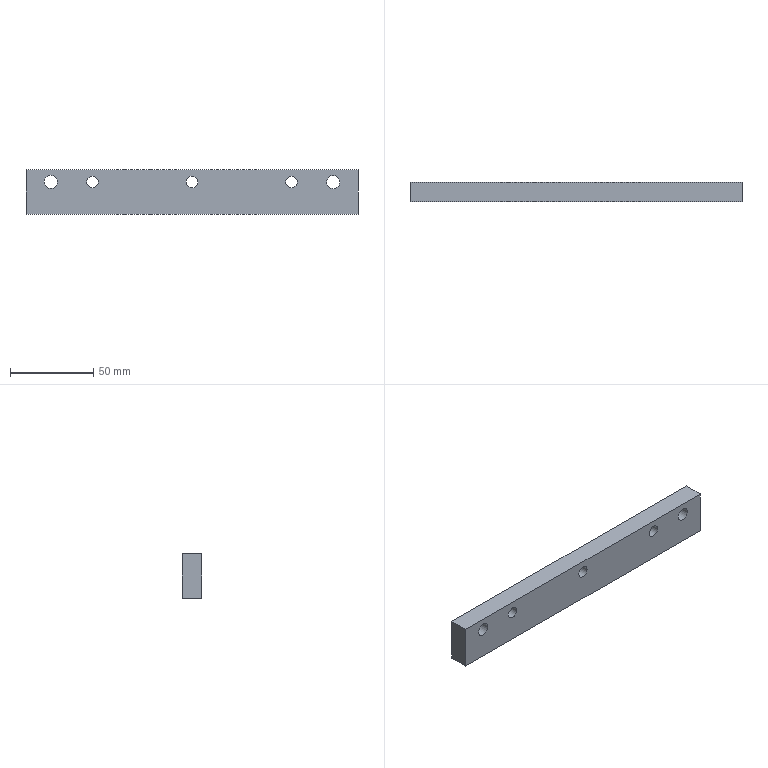Part | STEP file | SN10_001_003_GUIA | 1 solid | 17 faces | box 200 x 11.9 x 27 mm | volume 60502 mm3 | plane 9 | cylinder 8 | commonest cylinder face diameters 7 x3 11 x3 8 x2
STEP:
#1=CARTESIAN_POINT('',(0.,0.,0.));
#2=DIRECTION('',(0.,0.,1.));
#3=DIRECTION('',(1.,0.,0.));
#4=AXIS2_PLACEMENT_3D('',#1,#2,#3);
#5=CARTESIAN_POINT('',(88.51,226.9,59.418));
#6=VERTEX_POINT('',#5);
#7=CARTESIAN_POINT('',(85.,226.9,57.5));
#8=DIRECTION('',(0.,-1.,0.));
#9=DIRECTION('',(1.,0.,0.));
#10=AXIS2_PLACEMENT_3D('',#7,#8,#9);
#11=CIRCLE('',#10,4.);
#12=CARTESIAN_POINT('',(85.,226.8,57.5));
#13=DIRECTION('',(0.,-1.,0.));
#14=DIRECTION('',(0.8776,0.,0.4794));
#15=AXIS2_PLACEMENT_3D('',#12,#13,#14);
#16=CYLINDRICAL_SURFACE('',#15,4.);
#17=CARTESIAN_POINT('',(-0.5,-0.1));
#18=DIRECTION('',(1.,0.));
#19=VECTOR('',#18,1.);
#20=LINE('',#17,#19);
#21=(GEOMETRIC_REPRESENTATION_CONTEXT(2)PARAMETRIC_REPRESENTATION_CONTEXT()REPRESENTATION_CONTEXT('',''));
#22=DEFINITIONAL_REPRESENTATION('',(#20),#21);
#23=PCURVE('',#16,#22);
#24=CARTESIAN_POINT('',(0.,226.9,65.));
#25=DIRECTION('',(0.,-1.,0.));
#26=DIRECTION('',(0.,0.,-1.));
#27=AXIS2_PLACEMENT_3D('',#24,#25,#26);
#28=PLANE('',#27);
#29=CARTESIAN_POINT('',(7.5,85.));
#30=DIRECTION('',(0.,1.));
#31=AXIS2_PLACEMENT_2D('',#29,#30);
#32=CIRCLE('',#31,4.);
#33=(GEOMETRIC_REPRESENTATION_CONTEXT(2)PARAMETRIC_REPRESENTATION_CONTEXT()REPRESENTATION_CONTEXT('',''));
#34=DEFINITIONAL_REPRESENTATION('',(#32),#33);
#35=PCURVE('',#28,#34);
#36=SURFACE_CURVE('',#11,(#23,#35),.PCURVE_S1.);
#37=EDGE_CURVE('',#6,#6,#36,.T.);
#38=ORIENTED_EDGE('',*,*,#37,.T.);
#39=CARTESIAN_POINT('',(88.51,215.,59.418));
#40=VERTEX_POINT('',#39);
#41=CARTESIAN_POINT('',(88.51,226.9,59.418));
#42=CARTESIAN_POINT('',(88.51,215.,59.418));
#43=B_SPLINE_CURVE_WITH_KNOTS('',1,(#41,#42),.UNSPECIFIED.,.F.,.F.,(2,2),(-0.1,11.8),.PIECEWISE_BEZIER_KNOTS.);
#44=CARTESIAN_POINT('',(6.283,0.));
#45=DIRECTION('',(0.,1.));
#46=VECTOR('',#45,1.);
#47=LINE('',#44,#46);
#48=(GEOMETRIC_REPRESENTATION_CONTEXT(2)PARAMETRIC_REPRESENTATION_CONTEXT()REPRESENTATION_CONTEXT('',''));
#49=DEFINITIONAL_REPRESENTATION('',(#47),#48);
#50=PCURVE('',#16,#49);
#51=CARTESIAN_POINT('',(0.,0.));
#52=DIRECTION('',(0.,1.));
#53=VECTOR('',#52,1.);
#54=LINE('',#51,#53);
#55=(GEOMETRIC_REPRESENTATION_CONTEXT(2)PARAMETRIC_REPRESENTATION_CONTEXT()REPRESENTATION_CONTEXT('',''));
#56=DEFINITIONAL_REPRESENTATION('',(#54),#55);
#57=PCURVE('',#16,#56);
#58=SEAM_CURVE('',#43,(#50,#57),.PCURVE_S1.);
#59=EDGE_CURVE('',#6,#40,#58,.T.);
#60=ORIENTED_EDGE('',*,*,#59,.T.);
#61=CARTESIAN_POINT('',(85.,215.,57.5));
#62=DIRECTION('',(0.,-1.,0.));
#63=DIRECTION('',(1.,0.,0.));
#64=AXIS2_PLACEMENT_3D('',#61,#62,#63);
#65=CIRCLE('',#64,4.);
#66=CARTESIAN_POINT('',(-0.5,11.8));
#67=DIRECTION('',(1.,0.));
#68=VECTOR('',#67,1.);
#69=LINE('',#66,#68);
#70=(GEOMETRIC_REPRESENTATION_CONTEXT(2)PARAMETRIC_REPRESENTATION_CONTEXT()REPRESENTATION_CONTEXT('',''));
#71=DEFINITIONAL_REPRESENTATION('',(#69),#70);
#72=PCURVE('',#16,#71);
#73=CARTESIAN_POINT('',(0.,215.,38.));
#74=DIRECTION('',(0.,1.,0.));
#75=DIRECTION('',(0.,0.,1.));
#76=AXIS2_PLACEMENT_3D('',#73,#74,#75);
#77=PLANE('',#76);
#78=CARTESIAN_POINT('',(19.5,89.));
#79=CARTESIAN_POINT('',(26.428,89.));
#80=CARTESIAN_POINT('',(22.964,83.));
#81=CARTESIAN_POINT('',(19.5,77.));
#82=CARTESIAN_POINT('',(16.036,83.));
#83=CARTESIAN_POINT('',(12.572,89.));
#84=CARTESIAN_POINT('',(19.5,89.));
#85=(BOUNDED_CURVE()B_SPLINE_CURVE(2,(#78,#79,#80,#81,#82,#83,#84),.UNSPECIFIED.,.T.,.F.)B_SPLINE_CURVE_WITH_KNOTS((1,2,2,2,2,1),(-2.094,0.,2.094,4.189,6.283,8.378),.UNSPECIFIED.)CURVE()GEOMETRIC_REPRESENTATION_ITEM()RATIONAL_B_SPLINE_CURVE((1.,0.5,1.,0.5,1.,0.5,1.))REPRESENTATION_ITEM(''));
#86=(GEOMETRIC_REPRESENTATION_CONTEXT(2)PARAMETRIC_REPRESENTATION_CONTEXT()REPRESENTATION_CONTEXT('',''));
#87=DEFINITIONAL_REPRESENTATION('',(#85),#86);
#88=PCURVE('',#77,#87);
#89=SURFACE_CURVE('',#65,(#72,#88),.PCURVE_S1.);
#90=EDGE_CURVE('',#40,#40,#89,.T.);
#91=ORIENTED_EDGE('',*,*,#90,.F.);
#92=ORIENTED_EDGE('',*,*,#59,.F.);
#93=EDGE_LOOP('',(#38,#60,#91,#92));
#94=FACE_BOUND('',#93,.F.);
#95=ADVANCED_FACE('',(#94),#16,.F.);
#96=CARTESIAN_POINT('',(-100.,226.9,65.));
#97=VERTEX_POINT('',#96);
#98=CARTESIAN_POINT('',(100.,226.9,65.));
#99=VERTEX_POINT('',#98);
#100=CARTESIAN_POINT('',(-100.,226.9,65.));
#101=DIRECTION('',(1.,0.,0.));
#102=VECTOR('',#101,1.);
#103=LINE('',#100,#102);
#104=CARTESIAN_POINT('',(0.,215.,65.));
#105=DIRECTION('',(0.,0.,-1.));
#106=DIRECTION('',(-1.,0.,0.));
#107=AXIS2_PLACEMENT_3D('',#104,#105,#106);
#108=PLANE('',#107);
#109=CARTESIAN_POINT('',(100.,11.9));
#110=DIRECTION('',(-1.,0.));
#111=VECTOR('',#110,1.);
#112=LINE('',#109,#111);
#113=(GEOMETRIC_REPRESENTATION_CONTEXT(2)PARAMETRIC_REPRESENTATION_CONTEXT()REPRESENTATION_CONTEXT('',''));
#114=DEFINITIONAL_REPRESENTATION('',(#112),#113);
#115=PCURVE('',#108,#114);
#116=CARTESIAN_POINT('',(0.,-100.));
#117=DIRECTION('',(0.,1.));
#118=VECTOR('',#117,1.);
#119=LINE('',#116,#118);
#120=(GEOMETRIC_REPRESENTATION_CONTEXT(2)PARAMETRIC_REPRESENTATION_CONTEXT()REPRESENTATION_CONTEXT('',''));
#121=DEFINITIONAL_REPRESENTATION('',(#119),#120);
#122=PCURVE('',#28,#121);
#123=SURFACE_CURVE('',#103,(#115,#122),.PCURVE_S1.);
#124=EDGE_CURVE('',#97,#99,#123,.T.);
#125=ORIENTED_EDGE('',*,*,#124,.F.);
#126=CARTESIAN_POINT('',(-100.,215.,65.));
#127=VERTEX_POINT('',#126);
#128=CARTESIAN_POINT('',(-100.,215.,65.));
#129=DIRECTION('',(0.,1.,0.));
#130=VECTOR('',#129,1.);
#131=LINE('',#128,#130);
#132=CARTESIAN_POINT('',(100.,0.));
#133=DIRECTION('',(0.,1.));
#134=VECTOR('',#133,1.);
#135=LINE('',#132,#134);
#136=(GEOMETRIC_REPRESENTATION_CONTEXT(2)PARAMETRIC_REPRESENTATION_CONTEXT()REPRESENTATION_CONTEXT('',''));
#137=DEFINITIONAL_REPRESENTATION('',(#135),#136);
#138=PCURVE('',#108,#137);
#139=CARTESIAN_POINT('',(-100.,0.,0.));
#140=DIRECTION('',(1.,0.,0.));
#141=DIRECTION('',(0.,0.,-1.));
#142=AXIS2_PLACEMENT_3D('',#139,#140,#141);
#143=PLANE('',#142);
#144=CARTESIAN_POINT('',(-65.,215.));
#145=DIRECTION('',(0.,1.));
#146=VECTOR('',#145,1.);
#147=LINE('',#144,#146);
#148=(GEOMETRIC_REPRESENTATION_CONTEXT(2)PARAMETRIC_REPRESENTATION_CONTEXT()REPRESENTATION_CONTEXT('',''));
#149=DEFINITIONAL_REPRESENTATION('',(#147),#148);
#150=PCURVE('',#143,#149);
#151=SURFACE_CURVE('',#131,(#138,#150),.PCURVE_S1.);
#152=EDGE_CURVE('',#127,#97,#151,.T.);
#153=ORIENTED_EDGE('',*,*,#152,.F.);
#154=CARTESIAN_POINT('',(100.,215.,65.));
#155=VERTEX_POINT('',#154);
#156=CARTESIAN_POINT('',(-100.,215.,65.));
#157=DIRECTION('',(1.,0.,0.));
#158=VECTOR('',#157,1.);
#159=LINE('',#156,#158);
#160=CARTESIAN_POINT('',(100.,0.));
#161=DIRECTION('',(-1.,0.));
#162=VECTOR('',#161,1.);
#163=LINE('',#160,#162);
#164=(GEOMETRIC_REPRESENTATION_CONTEXT(2)PARAMETRIC_REPRESENTATION_CONTEXT()REPRESENTATION_CONTEXT('',''));
#165=DEFINITIONAL_REPRESENTATION('',(#163),#164);
#166=PCURVE('',#108,#165);
#167=CARTESIAN_POINT('',(27.,-100.));
#168=DIRECTION('',(0.,1.));
#169=VECTOR('',#168,1.);
#170=LINE('',#167,#169);
#171=(GEOMETRIC_REPRESENTATION_CONTEXT(2)PARAMETRIC_REPRESENTATION_CONTEXT()REPRESENTATION_CONTEXT('',''));
#172=DEFINITIONAL_REPRESENTATION('',(#170),#171);
#173=PCURVE('',#77,#172);
#174=SURFACE_CURVE('',#159,(#166,#173),.PCURVE_S1.);
#175=EDGE_CURVE('',#127,#155,#174,.T.);
#176=ORIENTED_EDGE('',*,*,#175,.T.);
#177=CARTESIAN_POINT('',(100.,215.,65.));
#178=DIRECTION('',(0.,1.,0.));
#179=VECTOR('',#178,1.);
#180=LINE('',#177,#179);
#181=CARTESIAN_POINT('',(-100.,0.));
#182=DIRECTION('',(0.,1.));
#183=VECTOR('',#182,1.);
#184=LINE('',#181,#183);
#185=(GEOMETRIC_REPRESENTATION_CONTEXT(2)PARAMETRIC_REPRESENTATION_CONTEXT()REPRESENTATION_CONTEXT('',''));
#186=DEFINITIONAL_REPRESENTATION('',(#184),#185);
#187=PCURVE('',#108,#186);
#188=CARTESIAN_POINT('',(100.,0.,0.));
#189=DIRECTION('',(1.,0.,0.));
#190=DIRECTION('',(0.,0.,-1.));
#191=AXIS2_PLACEMENT_3D('',#188,#189,#190);
#192=PLANE('',#191);
#193=CARTESIAN_POINT('',(-65.,215.));
#194=DIRECTION('',(0.,1.));
#195=VECTOR('',#194,1.);
#196=LINE('',#193,#195);
#197=(GEOMETRIC_REPRESENTATION_CONTEXT(2)PARAMETRIC_REPRESENTATION_CONTEXT()REPRESENTATION_CONTEXT('',''));
#198=DEFINITIONAL_REPRESENTATION('',(#196),#197);
#199=PCURVE('',#192,#198);
#200=SURFACE_CURVE('',#180,(#187,#199),.PCURVE_S1.);
#201=EDGE_CURVE('',#155,#99,#200,.T.);
#202=ORIENTED_EDGE('',*,*,#201,.T.);
#203=EDGE_LOOP('',(#125,#153,#176,#202));
#204=FACE_BOUND('',#203,.T.);
#205=ADVANCED_FACE('',(#204),#108,.F.);
#206=CARTESIAN_POINT('',(-100.,226.9,38.));
#207=VERTEX_POINT('',#206);
#208=CARTESIAN_POINT('',(-100.,226.9,65.));
#209=DIRECTION('',(0.,0.,-1.));
#210=VECTOR('',#209,1.);
#211=LINE('',#208,#210);
#212=CARTESIAN_POINT('',(-65.,226.9));
#213=DIRECTION('',(1.,0.));
#214=VECTOR('',#213,1.);
#215=LINE('',#212,#214);
#216=(GEOMETRIC_REPRESENTATION_CONTEXT(2)PARAMETRIC_REPRESENTATION_CONTEXT()REPRESENTATION_CONTEXT('',''));
#217=DEFINITIONAL_REPRESENTATION('',(#215),#216);
#218=PCURVE('',#143,#217);
#219=CARTESIAN_POINT('',(0.,-100.));
#220=DIRECTION('',(1.,0.));
#221=VECTOR('',#220,1.);
#222=LINE('',#219,#221);
#223=(GEOMETRIC_REPRESENTATION_CONTEXT(2)PARAMETRIC_REPRESENTATION_CONTEXT()REPRESENTATION_CONTEXT('',''));
#224=DEFINITIONAL_REPRESENTATION('',(#222),#223);
#225=PCURVE('',#28,#224);
#226=SURFACE_CURVE('',#211,(#218,#225),.PCURVE_S1.);
#227=EDGE_CURVE('',#97,#207,#226,.T.);
#228=ORIENTED_EDGE('',*,*,#227,.T.);
#229=CARTESIAN_POINT('',(-100.,215.,38.));
#230=VERTEX_POINT('',#229);
#231=CARTESIAN_POINT('',(-100.,226.9,38.));
#232=DIRECTION('',(0.,-1.,0.));
#233=VECTOR('',#232,1.);
#234=LINE('',#231,#233);
#235=CARTESIAN_POINT('',(-38.,226.9));
#236=DIRECTION('',(0.,-1.));
#237=VECTOR('',#236,1.);
#238=LINE('',#235,#237);
#239=(GEOMETRIC_REPRESENTATION_CONTEXT(2)PARAMETRIC_REPRESENTATION_CONTEXT()REPRESENTATION_CONTEXT('',''));
#240=DEFINITIONAL_REPRESENTATION('',(#238),#239);
#241=PCURVE('',#143,#240);
#242=CARTESIAN_POINT('',(0.,226.9,38.));
#243=DIRECTION('',(0.,0.,1.));
#244=DIRECTION('',(1.,0.,0.));
#245=AXIS2_PLACEMENT_3D('',#242,#243,#244);
#246=PLANE('',#245);
#247=CARTESIAN_POINT('',(-100.,0.));
#248=DIRECTION('',(0.,-1.));
#249=VECTOR('',#248,1.);
#250=LINE('',#247,#249);
#251=(GEOMETRIC_REPRESENTATION_CONTEXT(2)PARAMETRIC_REPRESENTATION_CONTEXT()REPRESENTATION_CONTEXT('',''));
#252=DEFINITIONAL_REPRESENTATION('',(#250),#251);
#253=PCURVE('',#246,#252);
#254=SURFACE_CURVE('',#234,(#241,#253),.PCURVE_S1.);
#255=EDGE_CURVE('',#207,#230,#254,.T.);
#256=ORIENTED_EDGE('',*,*,#255,.T.);
#257=CARTESIAN_POINT('',(-100.,215.,38.));
#258=DIRECTION('',(0.,0.,1.));
#259=VECTOR('',#258,1.);
#260=LINE('',#257,#259);
#261=CARTESIAN_POINT('',(-38.,215.));
#262=DIRECTION('',(-1.,0.));
#263=VECTOR('',#262,1.);
#264=LINE('',#261,#263);
#265=(GEOMETRIC_REPRESENTATION_CONTEXT(2)PARAMETRIC_REPRESENTATION_CONTEXT()REPRESENTATION_CONTEXT('',''));
#266=DEFINITIONAL_REPRESENTATION('',(#264),#265);
#267=PCURVE('',#143,#266);
#268=CARTESIAN_POINT('',(0.,-100.));
#269=DIRECTION('',(1.,0.));
#270=VECTOR('',#269,1.);
#271=LINE('',#268,#270);
#272=(GEOMETRIC_REPRESENTATION_CONTEXT(2)PARAMETRIC_REPRESENTATION_CONTEXT()REPRESENTATION_CONTEXT('',''));
#273=DEFINITIONAL_REPRESENTATION('',(#271),#272);
#274=PCURVE('',#77,#273);
#275=SURFACE_CURVE('',#260,(#267,#274),.PCURVE_S1.);
#276=EDGE_CURVE('',#230,#127,#275,.T.);
#277=ORIENTED_EDGE('',*,*,#276,.T.);
#278=ORIENTED_EDGE('',*,*,#152,.T.);
#279=EDGE_LOOP('',(#228,#256,#277,#278));
#280=FACE_BOUND('',#279,.T.);
#281=ADVANCED_FACE('',(#280),#143,.F.);
#282=CARTESIAN_POINT('',(55.173,226.9,54.863));
#283=VERTEX_POINT('',#282);
#284=CARTESIAN_POINT('',(60.,226.9,57.5));
#285=DIRECTION('',(0.,-1.,0.));
#286=DIRECTION('',(1.,0.,0.));
#287=AXIS2_PLACEMENT_3D('',#284,#285,#286);
#288=CIRCLE('',#287,5.5);
#289=CARTESIAN_POINT('',(60.,226.8,57.5));
#290=DIRECTION('',(0.,-1.,0.));
#291=DIRECTION('',(0.8776,0.,0.4794));
#292=AXIS2_PLACEMENT_3D('',#289,#290,#291);
#293=CYLINDRICAL_SURFACE('',#292,5.5);
#294=CARTESIAN_POINT('',(-0.5,-0.1));
#295=DIRECTION('',(1.,0.));
#296=VECTOR('',#295,1.);
#297=LINE('',#294,#296);
#298=(GEOMETRIC_REPRESENTATION_CONTEXT(2)PARAMETRIC_REPRESENTATION_CONTEXT()REPRESENTATION_CONTEXT('',''));
#299=DEFINITIONAL_REPRESENTATION('',(#297),#298);
#300=PCURVE('',#293,#299);
#301=CARTESIAN_POINT('',(7.5,60.));
#302=DIRECTION('',(0.,1.));
#303=AXIS2_PLACEMENT_2D('',#301,#302);
#304=CIRCLE('',#303,5.5);
#305=(GEOMETRIC_REPRESENTATION_CONTEXT(2)PARAMETRIC_REPRESENTATION_CONTEXT()REPRESENTATION_CONTEXT('',''));
#306=DEFINITIONAL_REPRESENTATION('',(#304),#305);
#307=PCURVE('',#28,#306);
#308=SURFACE_CURVE('',#288,(#300,#307),.PCURVE_S1.);
#309=EDGE_CURVE('',#283,#283,#308,.T.);
#310=ORIENTED_EDGE('',*,*,#309,.T.);
#311=CARTESIAN_POINT('',(55.173,219.9,54.863));
#312=VERTEX_POINT('',#311);
#313=CARTESIAN_POINT('',(55.173,226.9,54.863));
#314=CARTESIAN_POINT('',(55.173,219.9,54.863));
#315=B_SPLINE_CURVE_WITH_KNOTS('',1,(#313,#314),.UNSPECIFIED.,.F.,.F.,(2,2),(-0.1,6.9),.PIECEWISE_BEZIER_KNOTS.);
#316=CARTESIAN_POINT('',(9.425,0.));
#317=DIRECTION('',(0.,1.));
#318=VECTOR('',#317,1.);
#319=LINE('',#316,#318);
#320=(GEOMETRIC_REPRESENTATION_CONTEXT(2)PARAMETRIC_REPRESENTATION_CONTEXT()REPRESENTATION_CONTEXT('',''));
#321=DEFINITIONAL_REPRESENTATION('',(#319),#320);
#322=PCURVE('',#293,#321);
#323=CARTESIAN_POINT('',(3.142,0.));
#324=DIRECTION('',(0.,1.));
#325=VECTOR('',#324,1.);
#326=LINE('',#323,#325);
#327=(GEOMETRIC_REPRESENTATION_CONTEXT(2)PARAMETRIC_REPRESENTATION_CONTEXT()REPRESENTATION_CONTEXT('',''));
#328=DEFINITIONAL_REPRESENTATION('',(#326),#327);
#329=PCURVE('',#293,#328);
#330=SEAM_CURVE('',#315,(#322,#329),.PCURVE_S1.);
#331=EDGE_CURVE('',#283,#312,#330,.T.);
#332=ORIENTED_EDGE('',*,*,#331,.T.);
#333=CARTESIAN_POINT('',(60.,219.9,57.5));
#334=DIRECTION('',(0.,-1.,0.));
#335=DIRECTION('',(1.,0.,0.));
#336=AXIS2_PLACEMENT_3D('',#333,#334,#335);
#337=CIRCLE('',#336,5.5);
#338=CARTESIAN_POINT('',(-0.5,6.9));
#339=DIRECTION('',(1.,0.));
#340=VECTOR('',#339,1.);
#341=LINE('',#338,#340);
#342=(GEOMETRIC_REPRESENTATION_CONTEXT(2)PARAMETRIC_REPRESENTATION_CONTEXT()REPRESENTATION_CONTEXT('',''));
#343=DEFINITIONAL_REPRESENTATION('',(#341),#342);
#344=PCURVE('',#293,#343);
#345=CARTESIAN_POINT('',(63.5,219.9,57.5));
#346=DIRECTION('',(0.,-1.,0.));
#347=DIRECTION('',(0.,0.,-1.));
#348=AXIS2_PLACEMENT_3D('',#345,#346,#347);
#349=PLANE('',#348);
#350=CARTESIAN_POINT('',(0.,-3.5));
#351=DIRECTION('',(0.,1.));
#352=AXIS2_PLACEMENT_2D('',#350,#351);
#353=CIRCLE('',#352,5.5);
#354=(GEOMETRIC_REPRESENTATION_CONTEXT(2)PARAMETRIC_REPRESENTATION_CONTEXT()REPRESENTATION_CONTEXT('',''));
#355=DEFINITIONAL_REPRESENTATION('',(#353),#354);
#356=PCURVE('',#349,#355);
#357=SURFACE_CURVE('',#337,(#344,#356),.PCURVE_S1.);
#358=EDGE_CURVE('',#312,#312,#357,.T.);
#359=ORIENTED_EDGE('',*,*,#358,.F.);
#360=ORIENTED_EDGE('',*,*,#331,.F.);
#361=EDGE_LOOP('',(#310,#332,#359,#360));
#362=FACE_BOUND('',#361,.F.);
#363=ADVANCED_FACE('',(#362),#293,.F.);
#364=CARTESIAN_POINT('',(-4.827,226.9,54.863));
#365=VERTEX_POINT('',#364);
#366=CARTESIAN_POINT('',(0.,226.9,57.5));
#367=DIRECTION('',(0.,-1.,0.));
#368=DIRECTION('',(1.,0.,0.));
#369=AXIS2_PLACEMENT_3D('',#366,#367,#368);
#370=CIRCLE('',#369,5.5);
#371=CARTESIAN_POINT('',(0.,226.8,57.5));
#372=DIRECTION('',(0.,-1.,0.));
#373=DIRECTION('',(0.8776,0.,0.4794));
#374=AXIS2_PLACEMENT_3D('',#371,#372,#373);
#375=CYLINDRICAL_SURFACE('',#374,5.5);
#376=CARTESIAN_POINT('',(-0.5,-0.1));
#377=DIRECTION('',(1.,0.));
#378=VECTOR('',#377,1.);
#379=LINE('',#376,#378);
#380=(GEOMETRIC_REPRESENTATION_CONTEXT(2)PARAMETRIC_REPRESENTATION_CONTEXT()REPRESENTATION_CONTEXT('',''));
#381=DEFINITIONAL_REPRESENTATION('',(#379),#380);
#382=PCURVE('',#375,#381);
#383=CARTESIAN_POINT('',(7.5,0.));
#384=DIRECTION('',(0.,1.));
#385=AXIS2_PLACEMENT_2D('',#383,#384);
#386=CIRCLE('',#385,5.5);
#387=(GEOMETRIC_REPRESENTATION_CONTEXT(2)PARAMETRIC_REPRESENTATION_CONTEXT()REPRESENTATION_CONTEXT('',''));
#388=DEFINITIONAL_REPRESENTATION('',(#386),#387);
#389=PCURVE('',#28,#388);
#390=SURFACE_CURVE('',#370,(#382,#389),.PCURVE_S1.);
#391=EDGE_CURVE('',#365,#365,#390,.T.);
#392=ORIENTED_EDGE('',*,*,#391,.T.);
#393=CARTESIAN_POINT('',(-4.827,219.9,54.863));
#394=VERTEX_POINT('',#393);
#395=CARTESIAN_POINT('',(-4.827,226.9,54.863));
#396=CARTESIAN_POINT('',(-4.827,219.9,54.863));
#397=B_SPLINE_CURVE_WITH_KNOTS('',1,(#395,#396),.UNSPECIFIED.,.F.,.F.,(2,2),(-0.1,6.9),.PIECEWISE_BEZIER_KNOTS.);
#398=CARTESIAN_POINT('',(9.425,0.));
#399=DIRECTION('',(0.,1.));
#400=VECTOR('',#399,1.);
#401=LINE('',#398,#400);
#402=(GEOMETRIC_REPRESENTATION_CONTEXT(2)PARAMETRIC_REPRESENTATION_CONTEXT()REPRESENTATION_CONTEXT('',''));
#403=DEFINITIONAL_REPRESENTATION('',(#401),#402);
#404=PCURVE('',#375,#403);
#405=CARTESIAN_POINT('',(3.142,0.));
#406=DIRECTION('',(0.,1.));
#407=VECTOR('',#406,1.);
#408=LINE('',#405,#407);
#409=(GEOMETRIC_REPRESENTATION_CONTEXT(2)PARAMETRIC_REPRESENTATION_CONTEXT()REPRESENTATION_CONTEXT('',''));
#410=DEFINITIONAL_REPRESENTATION('',(#408),#409);
#411=PCURVE('',#375,#410);
#412=SEAM_CURVE('',#397,(#404,#411),.PCURVE_S1.);
#413=EDGE_CURVE('',#365,#394,#412,.T.);
#414=ORIENTED_EDGE('',*,*,#413,.T.);
#415=CARTESIAN_POINT('',(0.,219.9,57.5));
#416=DIRECTION('',(0.,-1.,0.));
#417=DIRECTION('',(1.,0.,0.));
#418=AXIS2_PLACEMENT_3D('',#415,#416,#417);
#419=CIRCLE('',#418,5.5);
#420=CARTESIAN_POINT('',(-0.5,6.9));
#421=DIRECTION('',(1.,0.));
#422=VECTOR('',#421,1.);
#423=LINE('',#420,#422);
#424=(GEOMETRIC_REPRESENTATION_CONTEXT(2)PARAMETRIC_REPRESENTATION_CONTEXT()REPRESENTATION_CONTEXT('',''));
#425=DEFINITIONAL_REPRESENTATION('',(#423),#424);
#426=PCURVE('',#375,#425);
#427=CARTESIAN_POINT('',(63.5,219.9,57.5));
#428=DIRECTION('',(0.,-1.,0.));
#429=DIRECTION('',(0.,0.,-1.));
#430=AXIS2_PLACEMENT_3D('',#427,#428,#429);
#431=PLANE('',#430);
#432=CARTESIAN_POINT('',(0.,-63.5));
#433=DIRECTION('',(0.,1.));
#434=AXIS2_PLACEMENT_2D('',#432,#433);
#435=CIRCLE('',#434,5.5);
#436=(GEOMETRIC_REPRESENTATION_CONTEXT(2)PARAMETRIC_REPRESENTATION_CONTEXT()REPRESENTATION_CONTEXT('',''));
#437=DEFINITIONAL_REPRESENTATION('',(#435),#436);
#438=PCURVE('',#431,#437);
#439=SURFACE_CURVE('',#419,(#426,#438),.PCURVE_S1.);
#440=EDGE_CURVE('',#394,#394,#439,.T.);
#441=ORIENTED_EDGE('',*,*,#440,.F.);
#442=ORIENTED_EDGE('',*,*,#413,.F.);
#443=EDGE_LOOP('',(#392,#414,#441,#442));
#444=FACE_BOUND('',#443,.F.);
#445=ADVANCED_FACE('',(#444),#375,.F.);
#446=CARTESIAN_POINT('',(-64.827,226.9,54.863));
#447=VERTEX_POINT('',#446);
#448=CARTESIAN_POINT('',(-60.,226.9,57.5));
#449=DIRECTION('',(0.,-1.,0.));
#450=DIRECTION('',(1.,0.,0.));
#451=AXIS2_PLACEMENT_3D('',#448,#449,#450);
#452=CIRCLE('',#451,5.5);
#453=CARTESIAN_POINT('',(-60.,226.8,57.5));
#454=DIRECTION('',(0.,-1.,0.));
#455=DIRECTION('',(0.8776,0.,0.4794));
#456=AXIS2_PLACEMENT_3D('',#453,#454,#455);
#457=CYLINDRICAL_SURFACE('',#456,5.5);
#458=CARTESIAN_POINT('',(-0.5,-0.1));
#459=DIRECTION('',(1.,0.));
#460=VECTOR('',#459,1.);
#461=LINE('',#458,#460);
#462=(GEOMETRIC_REPRESENTATION_CONTEXT(2)PARAMETRIC_REPRESENTATION_CONTEXT()REPRESENTATION_CONTEXT('',''));
#463=DEFINITIONAL_REPRESENTATION('',(#461),#462);
#464=PCURVE('',#457,#463);
#465=CARTESIAN_POINT('',(7.5,-60.));
#466=DIRECTION('',(0.,1.));
#467=AXIS2_PLACEMENT_2D('',#465,#466);
#468=CIRCLE('',#467,5.5);
#469=(GEOMETRIC_REPRESENTATION_CONTEXT(2)PARAMETRIC_REPRESENTATION_CONTEXT()REPRESENTATION_CONTEXT('',''));
#470=DEFINITIONAL_REPRESENTATION('',(#468),#469);
#471=PCURVE('',#28,#470);
#472=SURFACE_CURVE('',#452,(#464,#471),.PCURVE_S1.);
#473=EDGE_CURVE('',#447,#447,#472,.T.);
#474=ORIENTED_EDGE('',*,*,#473,.T.);
#475=CARTESIAN_POINT('',(-64.827,219.9,54.863));
#476=VERTEX_POINT('',#475);
#477=CARTESIAN_POINT('',(-64.827,226.9,54.863));
#478=CARTESIAN_POINT('',(-64.827,219.9,54.863));
#479=B_SPLINE_CURVE_WITH_KNOTS('',1,(#477,#478),.UNSPECIFIED.,.F.,.F.,(2,2),(-0.1,6.9),.PIECEWISE_BEZIER_KNOTS.);
#480=CARTESIAN_POINT('',(9.425,0.));
#481=DIRECTION('',(0.,1.));
#482=VECTOR('',#481,1.);
#483=LINE('',#480,#482);
#484=(GEOMETRIC_REPRESENTATION_CONTEXT(2)PARAMETRIC_REPRESENTATION_CONTEXT()REPRESENTATION_CONTEXT('',''));
#485=DEFINITIONAL_REPRESENTATION('',(#483),#484);
#486=PCURVE('',#457,#485);
#487=CARTESIAN_POINT('',(3.142,0.));
#488=DIRECTION('',(0.,1.));
#489=VECTOR('',#488,1.);
#490=LINE('',#487,#489);
#491=(GEOMETRIC_REPRESENTATION_CONTEXT(2)PARAMETRIC_REPRESENTATION_CONTEXT()REPRESENTATION_CONTEXT('',''));
#492=DEFINITIONAL_REPRESENTATION('',(#490),#491);
#493=PCURVE('',#457,#492);
#494=SEAM_CURVE('',#479,(#486,#493),.PCURVE_S1.);
#495=EDGE_CURVE('',#447,#476,#494,.T.);
#496=ORIENTED_EDGE('',*,*,#495,.T.);
#497=CARTESIAN_POINT('',(-60.,219.9,57.5));
#498=DIRECTION('',(0.,-1.,0.));
#499=DIRECTION('',(1.,0.,0.));
#500=AXIS2_PLACEMENT_3D('',#497,#498,#499);
#501=CIRCLE('',#500,5.5);
#502=CARTESIAN_POINT('',(-0.5,6.9));
#503=DIRECTION('',(1.,0.));
#504=VECTOR('',#503,1.);
#505=LINE('',#502,#504);
#506=(GEOMETRIC_REPRESENTATION_CONTEXT(2)PARAMETRIC_REPRESENTATION_CONTEXT()REPRESENTATION_CONTEXT('',''));
#507=DEFINITIONAL_REPRESENTATION('',(#505),#506);
#508=PCURVE('',#457,#507);
#509=CARTESIAN_POINT('',(63.5,219.9,57.5));
#510=DIRECTION('',(0.,-1.,0.));
#511=DIRECTION('',(0.,0.,-1.));
#512=AXIS2_PLACEMENT_3D('',#509,#510,#511);
#513=PLANE('',#512);
#514=CARTESIAN_POINT('',(0.,-123.5));
#515=DIRECTION('',(0.,1.));
#516=AXIS2_PLACEMENT_2D('',#514,#515);
#517=CIRCLE('',#516,5.5);
#518=(GEOMETRIC_REPRESENTATION_CONTEXT(2)PARAMETRIC_REPRESENTATION_CONTEXT()REPRESENTATION_CONTEXT('',''));
#519=DEFINITIONAL_REPRESENTATION('',(#517),#518);
#520=PCURVE('',#513,#519);
#521=SURFACE_CURVE('',#501,(#508,#520),.PCURVE_S1.);
#522=EDGE_CURVE('',#476,#476,#521,.T.);
#523=ORIENTED_EDGE('',*,*,#522,.F.);
#524=ORIENTED_EDGE('',*,*,#495,.F.);
#525=EDGE_LOOP('',(#474,#496,#523,#524));
#526=FACE_BOUND('',#525,.F.);
#527=ADVANCED_FACE('',(#526),#457,.F.);
#528=ORIENTED_EDGE('',*,*,#358,.F.);
#529=EDGE_LOOP('',(#528));
#530=FACE_BOUND('',#529,.T.);
#531=CARTESIAN_POINT('',(63.072,219.9,59.178));
#532=VERTEX_POINT('',#531);
#533=CARTESIAN_POINT('',(60.,219.9,57.5));
#534=DIRECTION('',(0.,-1.,0.));
#535=DIRECTION('',(1.,0.,0.));
#536=AXIS2_PLACEMENT_3D('',#533,#534,#535);
#537=CIRCLE('',#536,3.5);
#538=CARTESIAN_POINT('',(0.,-3.5));
#539=DIRECTION('',(0.,1.));
#540=AXIS2_PLACEMENT_2D('',#538,#539);
#541=CIRCLE('',#540,3.5);
#542=(GEOMETRIC_REPRESENTATION_CONTEXT(2)PARAMETRIC_REPRESENTATION_CONTEXT()REPRESENTATION_CONTEXT('',''));
#543=DEFINITIONAL_REPRESENTATION('',(#541),#542);
#544=PCURVE('',#349,#543);
#545=CARTESIAN_POINT('',(60.,226.8,57.5));
#546=DIRECTION('',(0.,-1.,0.));
#547=DIRECTION('',(0.8776,0.,0.4794));
#548=AXIS2_PLACEMENT_3D('',#545,#546,#547);
#549=CYLINDRICAL_SURFACE('',#548,3.5);
#550=CARTESIAN_POINT('',(-0.5,6.9));
#551=DIRECTION('',(1.,0.));
#552=VECTOR('',#551,1.);
#553=LINE('',#550,#552);
#554=(GEOMETRIC_REPRESENTATION_CONTEXT(2)PARAMETRIC_REPRESENTATION_CONTEXT()REPRESENTATION_CONTEXT('',''));
#555=DEFINITIONAL_REPRESENTATION('',(#553),#554);
#556=PCURVE('',#549,#555);
#557=SURFACE_CURVE('',#537,(#544,#556),.PCURVE_S1.);
#558=EDGE_CURVE('',#532,#532,#557,.T.);
#559=ORIENTED_EDGE('',*,*,#558,.T.);
#560=EDGE_LOOP('',(#559));
#561=FACE_BOUND('',#560,.T.);
#562=ADVANCED_FACE('',(#530,#561),#349,.F.);
#563=ORIENTED_EDGE('',*,*,#440,.F.);
#564=EDGE_LOOP('',(#563));
#565=FACE_BOUND('',#564,.T.);
#566=CARTESIAN_POINT('',(3.072,219.9,59.178));
#567=VERTEX_POINT('',#566);
#568=CARTESIAN_POINT('',(0.,219.9,57.5));
#569=DIRECTION('',(0.,-1.,0.));
#570=DIRECTION('',(1.,0.,0.));
#571=AXIS2_PLACEMENT_3D('',#568,#569,#570);
#572=CIRCLE('',#571,3.5);
#573=CARTESIAN_POINT('',(0.,-63.5));
#574=DIRECTION('',(0.,1.));
#575=AXIS2_PLACEMENT_2D('',#573,#574);
#576=CIRCLE('',#575,3.5);
#577=(GEOMETRIC_REPRESENTATION_CONTEXT(2)PARAMETRIC_REPRESENTATION_CONTEXT()REPRESENTATION_CONTEXT('',''));
#578=DEFINITIONAL_REPRESENTATION('',(#576),#577);
#579=PCURVE('',#431,#578);
#580=CARTESIAN_POINT('',(0.,226.8,57.5));
#581=DIRECTION('',(0.,-1.,0.));
#582=DIRECTION('',(0.8776,0.,0.4794));
#583=AXIS2_PLACEMENT_3D('',#580,#581,#582);
#584=CYLINDRICAL_SURFACE('',#583,3.5);
#585=CARTESIAN_POINT('',(-0.5,6.9));
#586=DIRECTION('',(1.,0.));
#587=VECTOR('',#586,1.);
#588=LINE('',#585,#587);
#589=(GEOMETRIC_REPRESENTATION_CONTEXT(2)PARAMETRIC_REPRESENTATION_CONTEXT()REPRESENTATION_CONTEXT('',''));
#590=DEFINITIONAL_REPRESENTATION('',(#588),#589);
#591=PCURVE('',#584,#590);
#592=SURFACE_CURVE('',#572,(#579,#591),.PCURVE_S1.);
#593=EDGE_CURVE('',#567,#567,#592,.T.);
#594=ORIENTED_EDGE('',*,*,#593,.T.);
#595=EDGE_LOOP('',(#594));
#596=FACE_BOUND('',#595,.T.);
#597=ADVANCED_FACE('',(#565,#596),#431,.F.);
#598=ORIENTED_EDGE('',*,*,#522,.F.);
#599=EDGE_LOOP('',(#598));
#600=FACE_BOUND('',#599,.T.);
#601=CARTESIAN_POINT('',(-56.928,219.9,59.178));
#602=VERTEX_POINT('',#601);
#603=CARTESIAN_POINT('',(-60.,219.9,57.5));
#604=DIRECTION('',(0.,-1.,0.));
#605=DIRECTION('',(1.,0.,0.));
#606=AXIS2_PLACEMENT_3D('',#603,#604,#605);
#607=CIRCLE('',#606,3.5);
#608=CARTESIAN_POINT('',(0.,-123.5));
#609=DIRECTION('',(0.,1.));
#610=AXIS2_PLACEMENT_2D('',#608,#609);
#611=CIRCLE('',#610,3.5);
#612=(GEOMETRIC_REPRESENTATION_CONTEXT(2)PARAMETRIC_REPRESENTATION_CONTEXT()REPRESENTATION_CONTEXT('',''));
#613=DEFINITIONAL_REPRESENTATION('',(#611),#612);
#614=PCURVE('',#513,#613);
#615=CARTESIAN_POINT('',(-60.,226.8,57.5));
#616=DIRECTION('',(0.,-1.,0.));
#617=DIRECTION('',(0.8776,0.,0.4794));
#618=AXIS2_PLACEMENT_3D('',#615,#616,#617);
#619=CYLINDRICAL_SURFACE('',#618,3.5);
#620=CARTESIAN_POINT('',(-0.5,6.9));
#621=DIRECTION('',(1.,0.));
#622=VECTOR('',#621,1.);
#623=LINE('',#620,#622);
#624=(GEOMETRIC_REPRESENTATION_CONTEXT(2)PARAMETRIC_REPRESENTATION_CONTEXT()REPRESENTATION_CONTEXT('',''));
#625=DEFINITIONAL_REPRESENTATION('',(#623),#624);
#626=PCURVE('',#619,#625);
#627=SURFACE_CURVE('',#607,(#614,#626),.PCURVE_S1.);
#628=EDGE_CURVE('',#602,#602,#627,.T.);
#629=ORIENTED_EDGE('',*,*,#628,.T.);
#630=EDGE_LOOP('',(#629));
#631=FACE_BOUND('',#630,.T.);
#632=ADVANCED_FACE('',(#600,#631),#513,.F.);
#633=CARTESIAN_POINT('',(63.072,215.,59.178));
#634=VERTEX_POINT('',#633);
#635=CARTESIAN_POINT('',(60.,215.,57.5));
#636=DIRECTION('',(0.,-1.,0.));
#637=DIRECTION('',(1.,0.,0.));
#638=AXIS2_PLACEMENT_3D('',#635,#636,#637);
#639=CIRCLE('',#638,3.5);
#640=CARTESIAN_POINT('',(-0.5,11.8));
#641=DIRECTION('',(1.,0.));
#642=VECTOR('',#641,1.);
#643=LINE('',#640,#642);
#644=(GEOMETRIC_REPRESENTATION_CONTEXT(2)PARAMETRIC_REPRESENTATION_CONTEXT()REPRESENTATION_CONTEXT('',''));
#645=DEFINITIONAL_REPRESENTATION('',(#643),#644);
#646=PCURVE('',#549,#645);
#647=CARTESIAN_POINT('',(19.5,63.5));
#648=CARTESIAN_POINT('',(25.562,63.5));
#649=CARTESIAN_POINT('',(22.531,58.25));
#650=CARTESIAN_POINT('',(19.5,53.));
#651=CARTESIAN_POINT('',(16.469,58.25));
#652=CARTESIAN_POINT('',(13.438,63.5));
#653=CARTESIAN_POINT('',(19.5,63.5));
#654=(BOUNDED_CURVE()B_SPLINE_CURVE(2,(#647,#648,#649,#650,#651,#652,#653),.UNSPECIFIED.,.T.,.F.)B_SPLINE_CURVE_WITH_KNOTS((1,2,2,2,2,1),(-2.094,0.,2.094,4.189,6.283,8.378),.UNSPECIFIED.)CURVE()GEOMETRIC_REPRESENTATION_ITEM()RATIONAL_B_SPLINE_CURVE((1.,0.5,1.,0.5,1.,0.5,1.))REPRESENTATION_ITEM(''));
#655=(GEOMETRIC_REPRESENTATION_CONTEXT(2)PARAMETRIC_REPRESENTATION_CONTEXT()REPRESENTATION_CONTEXT('',''));
#656=DEFINITIONAL_REPRESENTATION('',(#654),#655);
#657=PCURVE('',#77,#656);
#658=SURFACE_CURVE('',#639,(#646,#657),.PCURVE_S1.);
#659=EDGE_CURVE('',#634,#634,#658,.T.);
#660=ORIENTED_EDGE('',*,*,#659,.F.);
#661=CARTESIAN_POINT('',(63.072,219.9,59.178));
#662=CARTESIAN_POINT('',(63.072,215.,59.178));
#663=B_SPLINE_CURVE_WITH_KNOTS('',1,(#661,#662),.UNSPECIFIED.,.F.,.F.,(2,2),(6.9,11.8),.PIECEWISE_BEZIER_KNOTS.);
#664=CARTESIAN_POINT('',(0.,0.));
#665=DIRECTION('',(0.,1.));
#666=VECTOR('',#665,1.);
#667=LINE('',#664,#666);
#668=(GEOMETRIC_REPRESENTATION_CONTEXT(2)PARAMETRIC_REPRESENTATION_CONTEXT()REPRESENTATION_CONTEXT('',''));
#669=DEFINITIONAL_REPRESENTATION('',(#667),#668);
#670=PCURVE('',#549,#669);
#671=CARTESIAN_POINT('',(6.283,0.));
#672=DIRECTION('',(0.,1.));
#673=VECTOR('',#672,1.);
#674=LINE('',#671,#673);
#675=(GEOMETRIC_REPRESENTATION_CONTEXT(2)PARAMETRIC_REPRESENTATION_CONTEXT()REPRESENTATION_CONTEXT('',''));
#676=DEFINITIONAL_REPRESENTATION('',(#674),#675);
#677=PCURVE('',#549,#676);
#678=SEAM_CURVE('',#663,(#670,#677),.PCURVE_S1.);
#679=EDGE_CURVE('',#532,#634,#678,.T.);
#680=ORIENTED_EDGE('',*,*,#679,.F.);
#681=ORIENTED_EDGE('',*,*,#558,.T.);
#682=ORIENTED_EDGE('',*,*,#679,.T.);
#683=EDGE_LOOP('',(#660,#680,#681,#682));
#684=FACE_BOUND('',#683,.F.);
#685=ADVANCED_FACE('',(#684),#549,.F.);
#686=CARTESIAN_POINT('',(3.072,215.,59.178));
#687=VERTEX_POINT('',#686);
#688=CARTESIAN_POINT('',(0.,215.,57.5));
#689=DIRECTION('',(0.,-1.,0.));
#690=DIRECTION('',(1.,0.,0.));
#691=AXIS2_PLACEMENT_3D('',#688,#689,#690);
#692=CIRCLE('',#691,3.5);
#693=CARTESIAN_POINT('',(-0.5,11.8));
#694=DIRECTION('',(1.,0.));
#695=VECTOR('',#694,1.);
#696=LINE('',#693,#695);
#697=(GEOMETRIC_REPRESENTATION_CONTEXT(2)PARAMETRIC_REPRESENTATION_CONTEXT()REPRESENTATION_CONTEXT('',''));
#698=DEFINITIONAL_REPRESENTATION('',(#696),#697);
#699=PCURVE('',#584,#698);
#700=CARTESIAN_POINT('',(19.5,3.5));
#701=CARTESIAN_POINT('',(25.562,3.5));
#702=CARTESIAN_POINT('',(22.531,-1.75));
#703=CARTESIAN_POINT('',(19.5,-7.));
#704=CARTESIAN_POINT('',(16.469,-1.75));
#705=CARTESIAN_POINT('',(13.438,3.5));
#706=CARTESIAN_POINT('',(19.5,3.5));
#707=(BOUNDED_CURVE()B_SPLINE_CURVE(2,(#700,#701,#702,#703,#704,#705,#706),.UNSPECIFIED.,.T.,.F.)B_SPLINE_CURVE_WITH_KNOTS((1,2,2,2,2,1),(-2.094,0.,2.094,4.189,6.283,8.378),.UNSPECIFIED.)CURVE()GEOMETRIC_REPRESENTATION_ITEM()RATIONAL_B_SPLINE_CURVE((1.,0.5,1.,0.5,1.,0.5,1.))REPRESENTATION_ITEM(''));
#708=(GEOMETRIC_REPRESENTATION_CONTEXT(2)PARAMETRIC_REPRESENTATION_CONTEXT()REPRESENTATION_CONTEXT('',''));
#709=DEFINITIONAL_REPRESENTATION('',(#707),#708);
#710=PCURVE('',#77,#709);
#711=SURFACE_CURVE('',#692,(#699,#710),.PCURVE_S1.);
#712=EDGE_CURVE('',#687,#687,#711,.T.);
#713=ORIENTED_EDGE('',*,*,#712,.F.);
#714=CARTESIAN_POINT('',(3.072,219.9,59.178));
#715=CARTESIAN_POINT('',(3.072,215.,59.178));
#716=B_SPLINE_CURVE_WITH_KNOTS('',1,(#714,#715),.UNSPECIFIED.,.F.,.F.,(2,2),(6.9,11.8),.PIECEWISE_BEZIER_KNOTS.);
#717=CARTESIAN_POINT('',(0.,0.));
#718=DIRECTION('',(0.,1.));
#719=VECTOR('',#718,1.);
#720=LINE('',#717,#719);
#721=(GEOMETRIC_REPRESENTATION_CONTEXT(2)PARAMETRIC_REPRESENTATION_CONTEXT()REPRESENTATION_CONTEXT('',''));
#722=DEFINITIONAL_REPRESENTATION('',(#720),#721);
#723=PCURVE('',#584,#722);
#724=CARTESIAN_POINT('',(6.283,0.));
#725=DIRECTION('',(0.,1.));
#726=VECTOR('',#725,1.);
#727=LINE('',#724,#726);
#728=(GEOMETRIC_REPRESENTATION_CONTEXT(2)PARAMETRIC_REPRESENTATION_CONTEXT()REPRESENTATION_CONTEXT('',''));
#729=DEFINITIONAL_REPRESENTATION('',(#727),#728);
#730=PCURVE('',#584,#729);
#731=SEAM_CURVE('',#716,(#723,#730),.PCURVE_S1.);
#732=EDGE_CURVE('',#567,#687,#731,.T.);
#733=ORIENTED_EDGE('',*,*,#732,.F.);
#734=ORIENTED_EDGE('',*,*,#593,.T.);
#735=ORIENTED_EDGE('',*,*,#732,.T.);
#736=EDGE_LOOP('',(#713,#733,#734,#735));
#737=FACE_BOUND('',#736,.F.);
#738=ADVANCED_FACE('',(#737),#584,.F.);
#739=CARTESIAN_POINT('',(-56.928,215.,59.178));
#740=VERTEX_POINT('',#739);
#741=CARTESIAN_POINT('',(-60.,215.,57.5));
#742=DIRECTION('',(0.,-1.,0.));
#743=DIRECTION('',(1.,0.,0.));
#744=AXIS2_PLACEMENT_3D('',#741,#742,#743);
#745=CIRCLE('',#744,3.5);
#746=CARTESIAN_POINT('',(-0.5,11.8));
#747=DIRECTION('',(1.,0.));
#748=VECTOR('',#747,1.);
#749=LINE('',#746,#748);
#750=(GEOMETRIC_REPRESENTATION_CONTEXT(2)PARAMETRIC_REPRESENTATION_CONTEXT()REPRESENTATION_CONTEXT('',''));
#751=DEFINITIONAL_REPRESENTATION('',(#749),#750);
#752=PCURVE('',#619,#751);
#753=CARTESIAN_POINT('',(19.5,-56.5));
#754=CARTESIAN_POINT('',(25.562,-56.5));
#755=CARTESIAN_POINT('',(22.531,-61.75));
#756=CARTESIAN_POINT('',(19.5,-67.));
#757=CARTESIAN_POINT('',(16.469,-61.75));
#758=CARTESIAN_POINT('',(13.438,-56.5));
#759=CARTESIAN_POINT('',(19.5,-56.5));
#760=(BOUNDED_CURVE()B_SPLINE_CURVE(2,(#753,#754,#755,#756,#757,#758,#759),.UNSPECIFIED.,.T.,.F.)B_SPLINE_CURVE_WITH_KNOTS((1,2,2,2,2,1),(-2.094,0.,2.094,4.189,6.283,8.378),.UNSPECIFIED.)CURVE()GEOMETRIC_REPRESENTATION_ITEM()RATIONAL_B_SPLINE_CURVE((1.,0.5,1.,0.5,1.,0.5,1.))REPRESENTATION_ITEM(''));
#761=(GEOMETRIC_REPRESENTATION_CONTEXT(2)PARAMETRIC_REPRESENTATION_CONTEXT()REPRESENTATION_CONTEXT('',''));
#762=DEFINITIONAL_REPRESENTATION('',(#760),#761);
#763=PCURVE('',#77,#762);
#764=SURFACE_CURVE('',#745,(#752,#763),.PCURVE_S1.);
#765=EDGE_CURVE('',#740,#740,#764,.T.);
#766=ORIENTED_EDGE('',*,*,#765,.F.);
#767=CARTESIAN_POINT('',(-56.928,219.9,59.178));
#768=CARTESIAN_POINT('',(-56.928,215.,59.178));
#769=B_SPLINE_CURVE_WITH_KNOTS('',1,(#767,#768),.UNSPECIFIED.,.F.,.F.,(2,2),(6.9,11.8),.PIECEWISE_BEZIER_KNOTS.);
#770=CARTESIAN_POINT('',(0.,0.));
#771=DIRECTION('',(0.,1.));
#772=VECTOR('',#771,1.);
#773=LINE('',#770,#772);
#774=(GEOMETRIC_REPRESENTATION_CONTEXT(2)PARAMETRIC_REPRESENTATION_CONTEXT()REPRESENTATION_CONTEXT('',''));
#775=DEFINITIONAL_REPRESENTATION('',(#773),#774);
#776=PCURVE('',#619,#775);
#777=CARTESIAN_POINT('',(6.283,0.));
#778=DIRECTION('',(0.,1.));
#779=VECTOR('',#778,1.);
#780=LINE('',#777,#779);
#781=(GEOMETRIC_REPRESENTATION_CONTEXT(2)PARAMETRIC_REPRESENTATION_CONTEXT()REPRESENTATION_CONTEXT('',''));
#782=DEFINITIONAL_REPRESENTATION('',(#780),#781);
#783=PCURVE('',#619,#782);
#784=SEAM_CURVE('',#769,(#776,#783),.PCURVE_S1.);
#785=EDGE_CURVE('',#602,#740,#784,.T.);
#786=ORIENTED_EDGE('',*,*,#785,.F.);
#787=ORIENTED_EDGE('',*,*,#628,.T.);
#788=ORIENTED_EDGE('',*,*,#785,.T.);
#789=EDGE_LOOP('',(#766,#786,#787,#788));
#790=FACE_BOUND('',#789,.F.);
#791=ADVANCED_FACE('',(#790),#619,.F.);
#792=CARTESIAN_POINT('',(100.,215.,38.));
#793=VERTEX_POINT('',#792);
#794=CARTESIAN_POINT('',(-100.,215.,38.));
#795=DIRECTION('',(1.,0.,0.));
#796=VECTOR('',#795,1.);
#797=LINE('',#794,#796);
#798=CARTESIAN_POINT('',(-100.,-11.9));
#799=DIRECTION('',(1.,0.));
#800=VECTOR('',#799,1.);
#801=LINE('',#798,#800);
#802=(GEOMETRIC_REPRESENTATION_CONTEXT(2)PARAMETRIC_REPRESENTATION_CONTEXT()REPRESENTATION_CONTEXT('',''));
#803=DEFINITIONAL_REPRESENTATION('',(#801),#802);
#804=PCURVE('',#246,#803);
#805=CARTESIAN_POINT('',(0.,-100.));
#806=DIRECTION('',(0.,1.));
#807=VECTOR('',#806,1.);
#808=LINE('',#805,#807);
#809=(GEOMETRIC_REPRESENTATION_CONTEXT(2)PARAMETRIC_REPRESENTATION_CONTEXT()REPRESENTATION_CONTEXT('',''));
#810=DEFINITIONAL_REPRESENTATION('',(#808),#809);
#811=PCURVE('',#77,#810);
#812=SURFACE_CURVE('',#797,(#804,#811),.PCURVE_S1.);
#813=EDGE_CURVE('',#230,#793,#812,.T.);
#814=ORIENTED_EDGE('',*,*,#813,.F.);
#815=ORIENTED_EDGE('',*,*,#255,.F.);
#816=CARTESIAN_POINT('',(100.,226.9,38.));
#817=VERTEX_POINT('',#816);
#818=CARTESIAN_POINT('',(-100.,226.9,38.));
#819=DIRECTION('',(1.,0.,0.));
#820=VECTOR('',#819,1.);
#821=LINE('',#818,#820);
#822=CARTESIAN_POINT('',(-100.,0.));
#823=DIRECTION('',(1.,0.));
#824=VECTOR('',#823,1.);
#825=LINE('',#822,#824);
#826=(GEOMETRIC_REPRESENTATION_CONTEXT(2)PARAMETRIC_REPRESENTATION_CONTEXT()REPRESENTATION_CONTEXT('',''));
#827=DEFINITIONAL_REPRESENTATION('',(#825),#826);
#828=PCURVE('',#246,#827);
#829=CARTESIAN_POINT('',(27.,-100.));
#830=DIRECTION('',(0.,1.));
#831=VECTOR('',#830,1.);
#832=LINE('',#829,#831);
#833=(GEOMETRIC_REPRESENTATION_CONTEXT(2)PARAMETRIC_REPRESENTATION_CONTEXT()REPRESENTATION_CONTEXT('',''));
#834=DEFINITIONAL_REPRESENTATION('',(#832),#833);
#835=PCURVE('',#28,#834);
#836=SURFACE_CURVE('',#821,(#828,#835),.PCURVE_S1.);
#837=EDGE_CURVE('',#207,#817,#836,.T.);
#838=ORIENTED_EDGE('',*,*,#837,.T.);
#839=CARTESIAN_POINT('',(100.,226.9,38.));
#840=DIRECTION('',(0.,-1.,0.));
#841=VECTOR('',#840,1.);
#842=LINE('',#839,#841);
#843=CARTESIAN_POINT('',(100.,0.));
#844=DIRECTION('',(0.,-1.));
#845=VECTOR('',#844,1.);
#846=LINE('',#843,#845);
#847=(GEOMETRIC_REPRESENTATION_CONTEXT(2)PARAMETRIC_REPRESENTATION_CONTEXT()REPRESENTATION_CONTEXT('',''));
#848=DEFINITIONAL_REPRESENTATION('',(#846),#847);
#849=PCURVE('',#246,#848);
#850=CARTESIAN_POINT('',(-38.,226.9));
#851=DIRECTION('',(0.,-1.));
#852=VECTOR('',#851,1.);
#853=LINE('',#850,#852);
#854=(GEOMETRIC_REPRESENTATION_CONTEXT(2)PARAMETRIC_REPRESENTATION_CONTEXT()REPRESENTATION_CONTEXT('',''));
#855=DEFINITIONAL_REPRESENTATION('',(#853),#854);
#856=PCURVE('',#192,#855);
#857=SURFACE_CURVE('',#842,(#849,#856),.PCURVE_S1.);
#858=EDGE_CURVE('',#817,#793,#857,.T.);
#859=ORIENTED_EDGE('',*,*,#858,.T.);
#860=EDGE_LOOP('',(#814,#815,#838,#859));
#861=FACE_BOUND('',#860,.T.);
#862=ADVANCED_FACE('',(#861),#246,.F.);
#863=ORIENTED_EDGE('',*,*,#201,.F.);
#864=CARTESIAN_POINT('',(100.,215.,38.));
#865=DIRECTION('',(0.,0.,1.));
#866=VECTOR('',#865,1.);
#867=LINE('',#864,#866);
#868=CARTESIAN_POINT('',(-38.,215.));
#869=DIRECTION('',(-1.,0.));
#870=VECTOR('',#869,1.);
#871=LINE('',#868,#870);
#872=(GEOMETRIC_REPRESENTATION_CONTEXT(2)PARAMETRIC_REPRESENTATION_CONTEXT()REPRESENTATION_CONTEXT('',''));
#873=DEFINITIONAL_REPRESENTATION('',(#871),#872);
#874=PCURVE('',#192,#873);
#875=CARTESIAN_POINT('',(0.,100.));
#876=DIRECTION('',(1.,0.));
#877=VECTOR('',#876,1.);
#878=LINE('',#875,#877);
#879=(GEOMETRIC_REPRESENTATION_CONTEXT(2)PARAMETRIC_REPRESENTATION_CONTEXT()REPRESENTATION_CONTEXT('',''));
#880=DEFINITIONAL_REPRESENTATION('',(#878),#879);
#881=PCURVE('',#77,#880);
#882=SURFACE_CURVE('',#867,(#874,#881),.PCURVE_S1.);
#883=EDGE_CURVE('',#793,#155,#882,.T.);
#884=ORIENTED_EDGE('',*,*,#883,.F.);
#885=ORIENTED_EDGE('',*,*,#858,.F.);
#886=CARTESIAN_POINT('',(100.,226.9,65.));
#887=DIRECTION('',(0.,0.,-1.));
#888=VECTOR('',#887,1.);
#889=LINE('',#886,#888);
#890=CARTESIAN_POINT('',(-65.,226.9));
#891=DIRECTION('',(1.,0.));
#892=VECTOR('',#891,1.);
#893=LINE('',#890,#892);
#894=(GEOMETRIC_REPRESENTATION_CONTEXT(2)PARAMETRIC_REPRESENTATION_CONTEXT()REPRESENTATION_CONTEXT('',''));
#895=DEFINITIONAL_REPRESENTATION('',(#893),#894);
#896=PCURVE('',#192,#895);
#897=CARTESIAN_POINT('',(0.,100.));
#898=DIRECTION('',(1.,0.));
#899=VECTOR('',#898,1.);
#900=LINE('',#897,#899);
#901=(GEOMETRIC_REPRESENTATION_CONTEXT(2)PARAMETRIC_REPRESENTATION_CONTEXT()REPRESENTATION_CONTEXT('',''));
#902=DEFINITIONAL_REPRESENTATION('',(#900),#901);
#903=PCURVE('',#28,#902);
#904=SURFACE_CURVE('',#889,(#896,#903),.PCURVE_S1.);
#905=EDGE_CURVE('',#99,#817,#904,.T.);
#906=ORIENTED_EDGE('',*,*,#905,.F.);
#907=EDGE_LOOP('',(#863,#884,#885,#906));
#908=FACE_BOUND('',#907,.T.);
#909=ADVANCED_FACE('',(#908),#192,.T.);
#910=ORIENTED_EDGE('',*,*,#837,.F.);
#911=ORIENTED_EDGE('',*,*,#227,.F.);
#912=ORIENTED_EDGE('',*,*,#124,.T.);
#913=ORIENTED_EDGE('',*,*,#905,.T.);
#914=EDGE_LOOP('',(#910,#911,#912,#913));
#915=FACE_BOUND('',#914,.T.);
#916=CARTESIAN_POINT('',(-81.49,226.9,59.418));
#917=VERTEX_POINT('',#916);
#918=CARTESIAN_POINT('',(-85.,226.9,57.5));
#919=DIRECTION('',(0.,-1.,0.));
#920=DIRECTION('',(1.,0.,0.));
#921=AXIS2_PLACEMENT_3D('',#918,#919,#920);
#922=CIRCLE('',#921,4.);
#923=CARTESIAN_POINT('',(7.5,-85.));
#924=DIRECTION('',(0.,1.));
#925=AXIS2_PLACEMENT_2D('',#923,#924);
#926=CIRCLE('',#925,4.);
#927=(GEOMETRIC_REPRESENTATION_CONTEXT(2)PARAMETRIC_REPRESENTATION_CONTEXT()REPRESENTATION_CONTEXT('',''));
#928=DEFINITIONAL_REPRESENTATION('',(#926),#927);
#929=PCURVE('',#28,#928);
#930=CARTESIAN_POINT('',(-85.,226.8,57.5));
#931=DIRECTION('',(0.,-1.,0.));
#932=DIRECTION('',(0.8776,0.,0.4794));
#933=AXIS2_PLACEMENT_3D('',#930,#931,#932);
#934=CYLINDRICAL_SURFACE('',#933,4.);
#935=CARTESIAN_POINT('',(-0.5,-0.1));
#936=DIRECTION('',(1.,0.));
#937=VECTOR('',#936,1.);
#938=LINE('',#935,#937);
#939=(GEOMETRIC_REPRESENTATION_CONTEXT(2)PARAMETRIC_REPRESENTATION_CONTEXT()REPRESENTATION_CONTEXT('',''));
#940=DEFINITIONAL_REPRESENTATION('',(#938),#939);
#941=PCURVE('',#934,#940);
#942=SURFACE_CURVE('',#922,(#929,#941),.PCURVE_S1.);
#943=EDGE_CURVE('',#917,#917,#942,.T.);
#944=ORIENTED_EDGE('',*,*,#943,.T.);
#945=EDGE_LOOP('',(#944));
#946=FACE_BOUND('',#945,.T.);
#947=ORIENTED_EDGE('',*,*,#37,.T.);
#948=EDGE_LOOP('',(#947));
#949=FACE_BOUND('',#948,.T.);
#950=ORIENTED_EDGE('',*,*,#309,.T.);
#951=EDGE_LOOP('',(#950));
#952=FACE_BOUND('',#951,.T.);
#953=ORIENTED_EDGE('',*,*,#391,.T.);
#954=EDGE_LOOP('',(#953));
#955=FACE_BOUND('',#954,.T.);
#956=ORIENTED_EDGE('',*,*,#473,.T.);
#957=EDGE_LOOP('',(#956));
#958=FACE_BOUND('',#957,.T.);
#959=ADVANCED_FACE('',(#915,#946,#949,#952,#955,#958),#28,.F.);
#960=ORIENTED_EDGE('',*,*,#175,.F.);
#961=ORIENTED_EDGE('',*,*,#276,.F.);
#962=ORIENTED_EDGE('',*,*,#813,.T.);
#963=ORIENTED_EDGE('',*,*,#883,.T.);
#964=EDGE_LOOP('',(#960,#961,#962,#963));
#965=FACE_BOUND('',#964,.T.);
#966=CARTESIAN_POINT('',(-81.49,215.,59.418));
#967=VERTEX_POINT('',#966);
#968=CARTESIAN_POINT('',(-85.,215.,57.5));
#969=DIRECTION('',(0.,1.,0.));
#970=DIRECTION('',(1.,0.,0.));
#971=AXIS2_PLACEMENT_3D('',#968,#969,#970);
#972=CIRCLE('',#971,4.);
#973=CARTESIAN_POINT('',(19.5,-85.));
#974=DIRECTION('',(0.,1.));
#975=AXIS2_PLACEMENT_2D('',#973,#974);
#976=CIRCLE('',#975,4.);
#977=(GEOMETRIC_REPRESENTATION_CONTEXT(2)PARAMETRIC_REPRESENTATION_CONTEXT()REPRESENTATION_CONTEXT('',''));
#978=DEFINITIONAL_REPRESENTATION('',(#976),#977);
#979=PCURVE('',#77,#978);
#980=CARTESIAN_POINT('',(12.066,11.8));
#981=DIRECTION('',(-1.,0.));
#982=VECTOR('',#981,1.);
#983=LINE('',#980,#982);
#984=(GEOMETRIC_REPRESENTATION_CONTEXT(2)PARAMETRIC_REPRESENTATION_CONTEXT()REPRESENTATION_CONTEXT('',''));
#985=DEFINITIONAL_REPRESENTATION('',(#983),#984);
#986=PCURVE('',#934,#985);
#987=SURFACE_CURVE('',#972,(#979,#986),.PCURVE_S1.);
#988=EDGE_CURVE('',#967,#967,#987,.T.);
#989=ORIENTED_EDGE('',*,*,#988,.T.);
#990=EDGE_LOOP('',(#989));
#991=FACE_BOUND('',#990,.T.);
#992=ORIENTED_EDGE('',*,*,#90,.F.);
#993=EDGE_LOOP('',(#992));
#994=FACE_BOUND('',#993,.T.);
#995=ORIENTED_EDGE('',*,*,#659,.F.);
#996=EDGE_LOOP('',(#995));
#997=FACE_BOUND('',#996,.T.);
#998=ORIENTED_EDGE('',*,*,#712,.F.);
#999=EDGE_LOOP('',(#998));
#1000=FACE_BOUND('',#999,.T.);
#1001=ORIENTED_EDGE('',*,*,#765,.F.);
#1002=EDGE_LOOP('',(#1001));
#1003=FACE_BOUND('',#1002,.T.);
#1004=ADVANCED_FACE('',(#965,#991,#994,#997,#1000,#1003),#77,.F.);
#1005=ORIENTED_EDGE('',*,*,#943,.T.);
#1006=CARTESIAN_POINT('',(-81.49,226.9,59.418));
#1007=CARTESIAN_POINT('',(-81.49,215.,59.418));
#1008=B_SPLINE_CURVE_WITH_KNOTS('',1,(#1006,#1007),.UNSPECIFIED.,.F.,.F.,(2,2),(-0.1,11.8),.PIECEWISE_BEZIER_KNOTS.);
#1009=CARTESIAN_POINT('',(6.283,0.));
#1010=DIRECTION('',(0.,1.));
#1011=VECTOR('',#1010,1.);
#1012=LINE('',#1009,#1011);
#1013=(GEOMETRIC_REPRESENTATION_CONTEXT(2)PARAMETRIC_REPRESENTATION_CONTEXT()REPRESENTATION_CONTEXT('',''));
#1014=DEFINITIONAL_REPRESENTATION('',(#1012),#1013);
#1015=PCURVE('',#934,#1014);
#1016=CARTESIAN_POINT('',(0.,0.));
#1017=DIRECTION('',(0.,1.));
#1018=VECTOR('',#1017,1.);
#1019=LINE('',#1016,#1018);
#1020=(GEOMETRIC_REPRESENTATION_CONTEXT(2)PARAMETRIC_REPRESENTATION_CONTEXT()REPRESENTATION_CONTEXT('',''));
#1021=DEFINITIONAL_REPRESENTATION('',(#1019),#1020);
#1022=PCURVE('',#934,#1021);
#1023=SEAM_CURVE('',#1008,(#1015,#1022),.PCURVE_S1.);
#1024=EDGE_CURVE('',#917,#967,#1023,.T.);
#1025=ORIENTED_EDGE('',*,*,#1024,.T.);
#1026=ORIENTED_EDGE('',*,*,#988,.T.);
#1027=ORIENTED_EDGE('',*,*,#1024,.F.);
#1028=EDGE_LOOP('',(#1005,#1025,#1026,#1027));
#1029=FACE_BOUND('',#1028,.F.);
#1030=ADVANCED_FACE('',(#1029),#934,.F.);
#1031=CLOSED_SHELL('',(#95,#205,#281,#363,#445,#527,#562,#597,#632,#685,#738,#791,#862,#909,#959,#1004,#1030));
#1032=MANIFOLD_SOLID_BREP('',#1031);
#1033=(LENGTH_UNIT()NAMED_UNIT(*)SI_UNIT(.MILLI.,.METRE.));
#1034=UNCERTAINTY_MEASURE_WITH_UNIT(LENGTH_MEASURE(0.000005),#1033,'','');
#1035=(NAMED_UNIT(*)PLANE_ANGLE_UNIT()SI_UNIT($,.RADIAN.));
#1036=(NAMED_UNIT(*)SI_UNIT($,.STERADIAN.)SOLID_ANGLE_UNIT());
#1037=(GEOMETRIC_REPRESENTATION_CONTEXT(3)GLOBAL_UNCERTAINTY_ASSIGNED_CONTEXT((#1034))GLOBAL_UNIT_ASSIGNED_CONTEXT((#1033,#1035,#1036))REPRESENTATION_CONTEXT('',''));
#1038=ADVANCED_BREP_SHAPE_REPRESENTATION('',(#4,#1032),#1037);